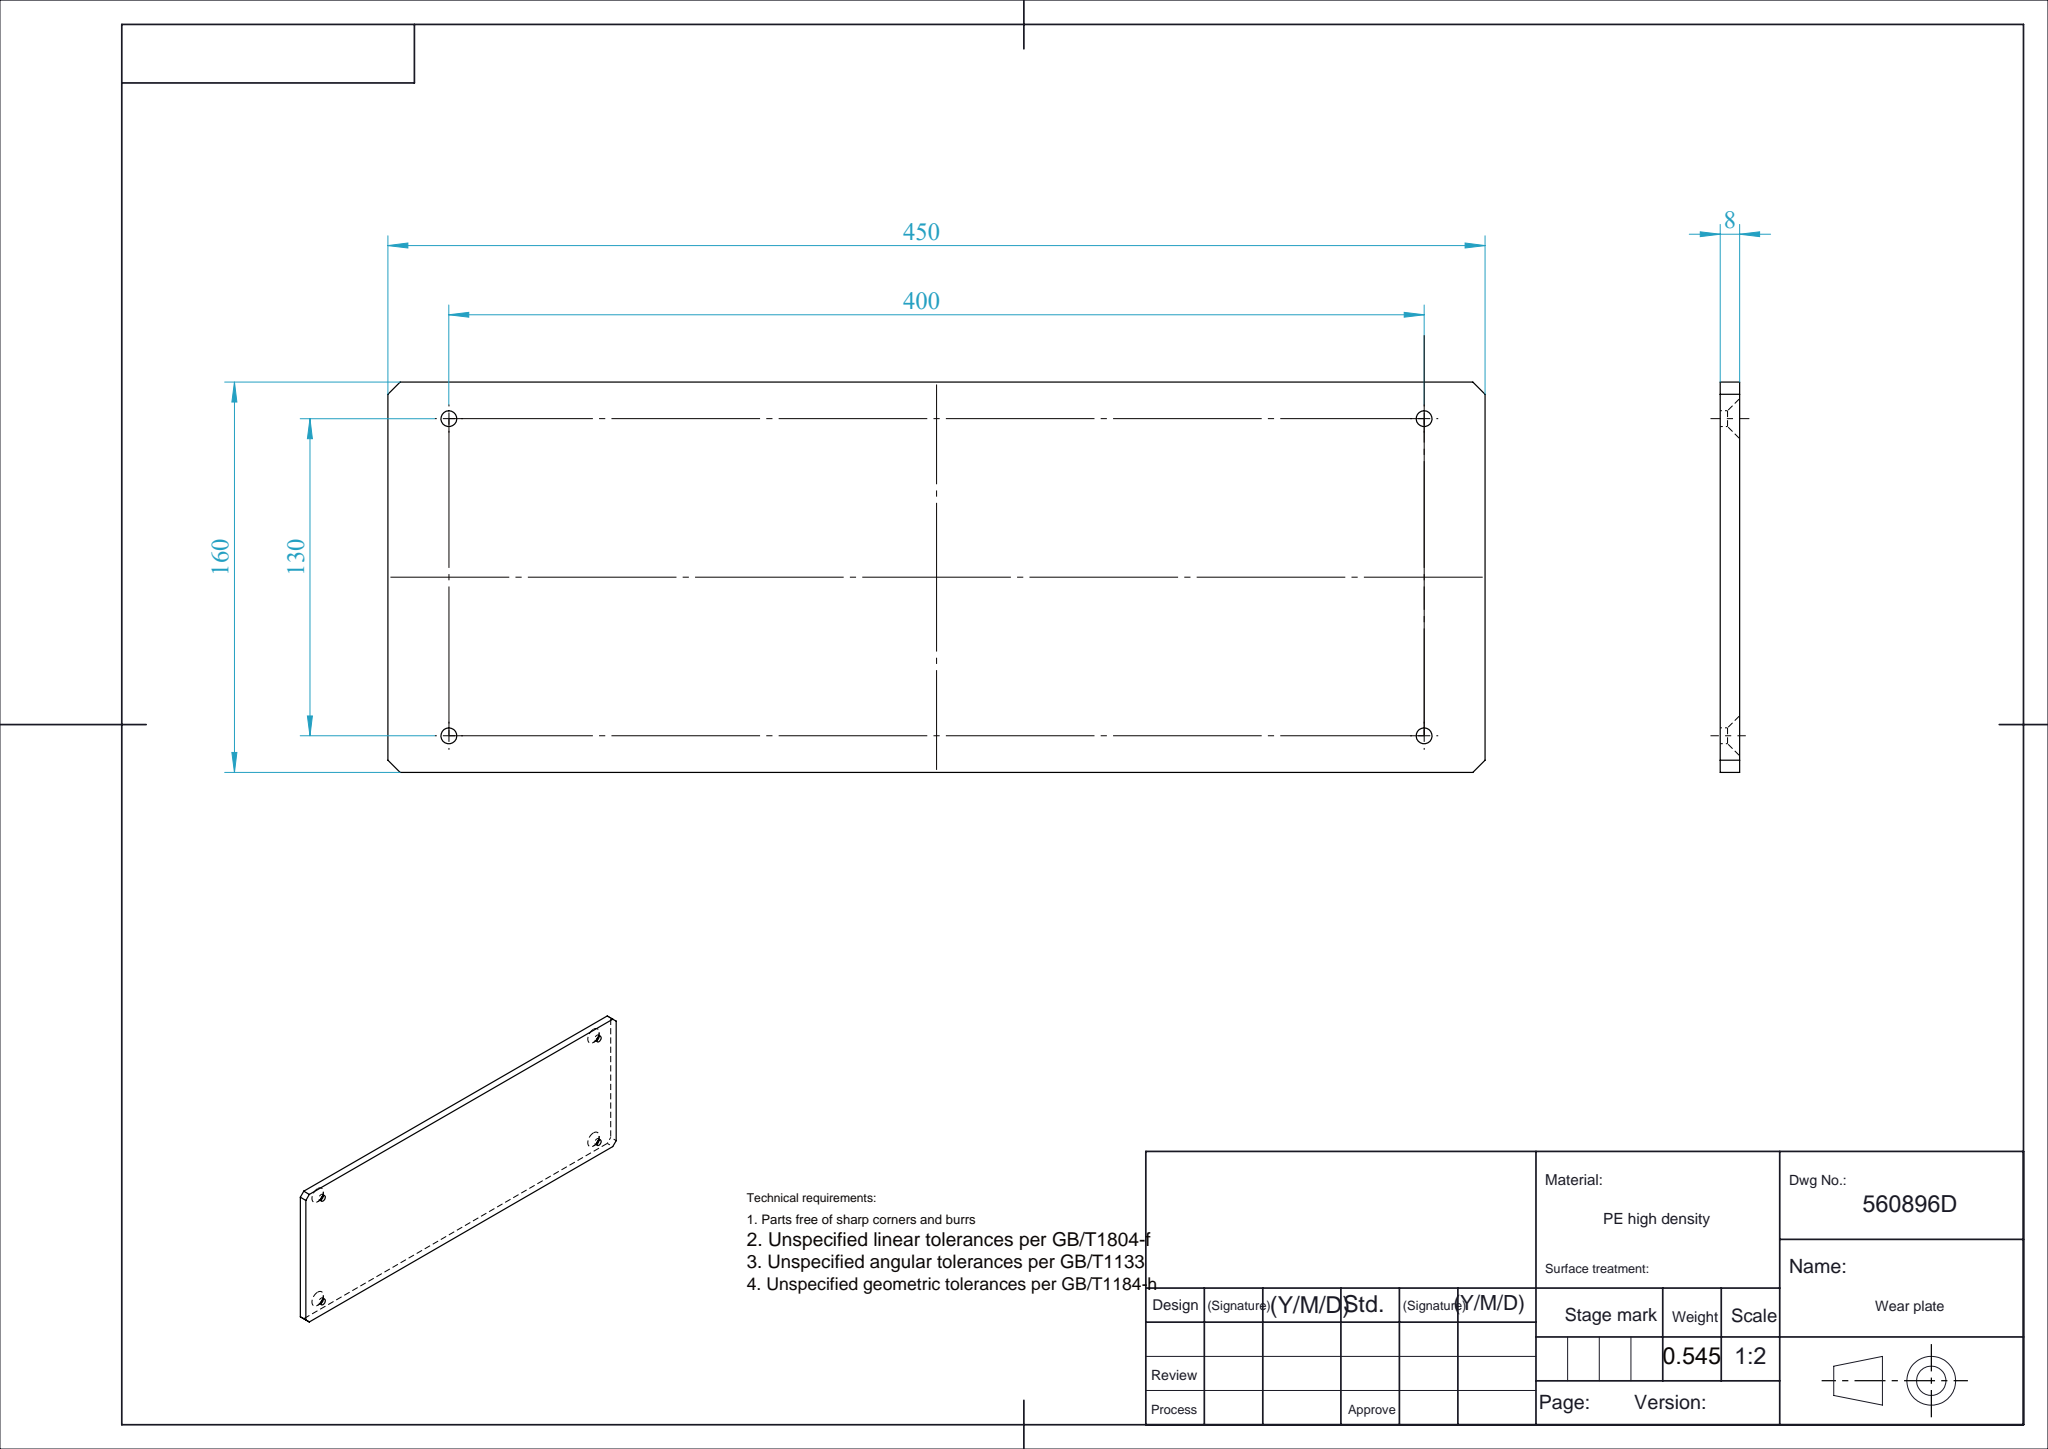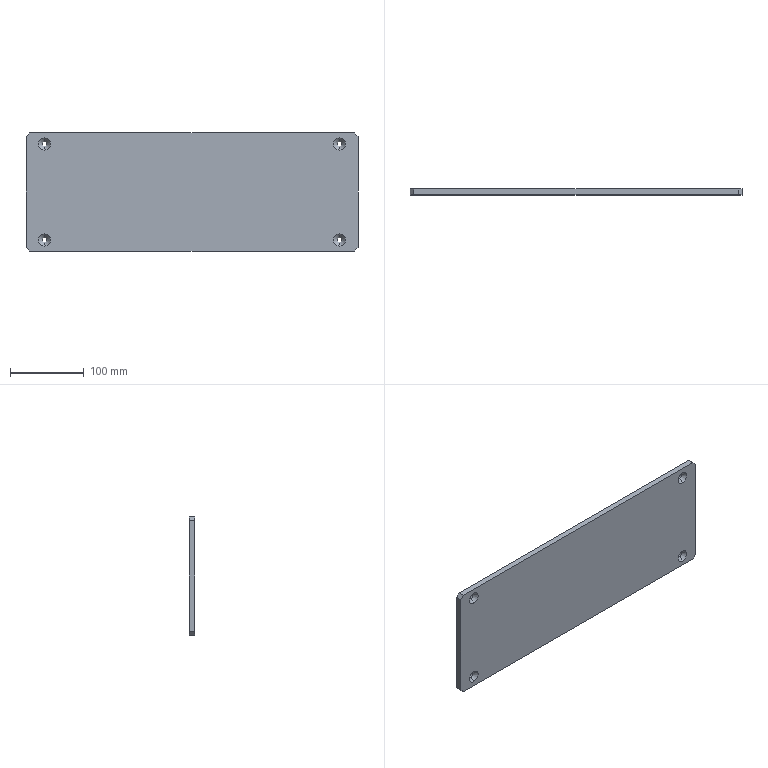Part | SolidWorks | features ICE 2, Chamfer 1, Extrusion 1 | 1 solid | 26 faces | box 450 x 8 x 160 mm | volume 572994 mm3 | plane 10 | cone 8 | cylinder 8 | commonest cylinder face diameters 6.5 x8
STEP:
#1=CARTESIAN_POINT('',(-200.,5.,68.25));
#2=VERTEX_POINT('',#1);
#3=CARTESIAN_POINT('',(-200.,5.,61.75));
#4=VERTEX_POINT('',#3);
#5=CARTESIAN_POINT('',(-200.,5.,65.));
#6=DIRECTION('',(0.,-1.,0.));
#7=DIRECTION('',(0.,0.,-1.));
#8=AXIS2_PLACEMENT_3D('',#5,#6,#7);
#9=CIRCLE('',#8,3.25);
#10=EDGE_CURVE('',#2,#4,#9,.T.);
#11=ORIENTED_EDGE('',*,*,#10,.F.);
#12=CARTESIAN_POINT('',(-200.,0.,73.25));
#13=VERTEX_POINT('',#12);
#14=CARTESIAN_POINT('',(-200.,0.,73.25));
#15=DIRECTION('',(0.,-0.7071,0.7071));
#16=VECTOR('',#15,1000.);
#17=LINE('',#14,#16);
#18=EDGE_CURVE('',#2,#13,#17,.T.);
#19=ORIENTED_EDGE('',*,*,#18,.T.);
#20=CARTESIAN_POINT('',(-200.,0.,56.75));
#21=VERTEX_POINT('',#20);
#22=CARTESIAN_POINT('',(-200.,0.,65.));
#23=DIRECTION('',(0.,-1.,0.));
#24=DIRECTION('',(0.,0.,-1.));
#25=AXIS2_PLACEMENT_3D('',#22,#23,#24);
#26=CIRCLE('',#25,8.25);
#27=EDGE_CURVE('',#13,#21,#26,.T.);
#28=ORIENTED_EDGE('',*,*,#27,.T.);
#29=CARTESIAN_POINT('',(-200.,0.,56.75));
#30=DIRECTION('',(0.,-0.7071,-0.7071));
#31=VECTOR('',#30,1000.);
#32=LINE('',#29,#31);
#33=EDGE_CURVE('',#4,#21,#32,.T.);
#34=ORIENTED_EDGE('',*,*,#33,.F.);
#35=EDGE_LOOP('',(#11,#19,#28,#34));
#36=FACE_OUTER_BOUND('',#35,.T.);
#37=CARTESIAN_POINT('',(-200.,0.,65.));
#38=DIRECTION('',(0.,-1.,0.));
#39=DIRECTION('',(0.,0.,-1.));
#40=AXIS2_PLACEMENT_3D('',#37,#38,#39);
#41=CONICAL_SURFACE('',#40,8.25,0.7854);
#42=ADVANCED_FACE('',(#36),#41,.F.);
#43=CARTESIAN_POINT('',(200.,5.,-61.75));
#44=VERTEX_POINT('',#43);
#45=CARTESIAN_POINT('',(200.,5.,-68.25));
#46=VERTEX_POINT('',#45);
#47=CARTESIAN_POINT('',(200.,5.,-65.));
#48=DIRECTION('',(0.,-1.,0.));
#49=DIRECTION('',(0.,0.,-1.));
#50=AXIS2_PLACEMENT_3D('',#47,#48,#49);
#51=CIRCLE('',#50,3.25);
#52=EDGE_CURVE('',#44,#46,#51,.T.);
#53=ORIENTED_EDGE('',*,*,#52,.F.);
#54=CARTESIAN_POINT('',(200.,0.,-56.75));
#55=VERTEX_POINT('',#54);
#56=CARTESIAN_POINT('',(200.,0.,-56.75));
#57=DIRECTION('',(0.,-0.7071,0.7071));
#58=VECTOR('',#57,1000.);
#59=LINE('',#56,#58);
#60=EDGE_CURVE('',#44,#55,#59,.T.);
#61=ORIENTED_EDGE('',*,*,#60,.T.);
#62=CARTESIAN_POINT('',(200.,0.,-73.25));
#63=VERTEX_POINT('',#62);
#64=CARTESIAN_POINT('',(200.,0.,-65.));
#65=DIRECTION('',(0.,-1.,0.));
#66=DIRECTION('',(0.,0.,-1.));
#67=AXIS2_PLACEMENT_3D('',#64,#65,#66);
#68=CIRCLE('',#67,8.25);
#69=EDGE_CURVE('',#55,#63,#68,.T.);
#70=ORIENTED_EDGE('',*,*,#69,.T.);
#71=CARTESIAN_POINT('',(200.,0.,-73.25));
#72=DIRECTION('',(0.,-0.7071,-0.7071));
#73=VECTOR('',#72,1000.);
#74=LINE('',#71,#73);
#75=EDGE_CURVE('',#46,#63,#74,.T.);
#76=ORIENTED_EDGE('',*,*,#75,.F.);
#77=EDGE_LOOP('',(#53,#61,#70,#76));
#78=FACE_OUTER_BOUND('',#77,.T.);
#79=CARTESIAN_POINT('',(200.,0.,-65.));
#80=DIRECTION('',(0.,-1.,0.));
#81=DIRECTION('',(0.,0.,-1.));
#82=AXIS2_PLACEMENT_3D('',#79,#80,#81);
#83=CONICAL_SURFACE('',#82,8.25,0.7854);
#84=ADVANCED_FACE('',(#78),#83,.F.);
#85=CARTESIAN_POINT('',(200.,5.,68.25));
#86=VERTEX_POINT('',#85);
#87=CARTESIAN_POINT('',(200.,5.,61.75));
#88=VERTEX_POINT('',#87);
#89=CARTESIAN_POINT('',(200.,5.,65.));
#90=DIRECTION('',(0.,-1.,0.));
#91=DIRECTION('',(0.,0.,-1.));
#92=AXIS2_PLACEMENT_3D('',#89,#90,#91);
#93=CIRCLE('',#92,3.25);
#94=EDGE_CURVE('',#86,#88,#93,.T.);
#95=ORIENTED_EDGE('',*,*,#94,.F.);
#96=CARTESIAN_POINT('',(200.,0.,73.25));
#97=VERTEX_POINT('',#96);
#98=CARTESIAN_POINT('',(200.,0.,73.25));
#99=DIRECTION('',(0.,-0.7071,0.7071));
#100=VECTOR('',#99,1000.);
#101=LINE('',#98,#100);
#102=EDGE_CURVE('',#86,#97,#101,.T.);
#103=ORIENTED_EDGE('',*,*,#102,.T.);
#104=CARTESIAN_POINT('',(200.,0.,56.75));
#105=VERTEX_POINT('',#104);
#106=CARTESIAN_POINT('',(200.,0.,65.));
#107=DIRECTION('',(0.,-1.,0.));
#108=DIRECTION('',(0.,0.,-1.));
#109=AXIS2_PLACEMENT_3D('',#106,#107,#108);
#110=CIRCLE('',#109,8.25);
#111=EDGE_CURVE('',#97,#105,#110,.T.);
#112=ORIENTED_EDGE('',*,*,#111,.T.);
#113=CARTESIAN_POINT('',(200.,0.,56.75));
#114=DIRECTION('',(0.,-0.7071,-0.7071));
#115=VECTOR('',#114,1000.);
#116=LINE('',#113,#115);
#117=EDGE_CURVE('',#88,#105,#116,.T.);
#118=ORIENTED_EDGE('',*,*,#117,.F.);
#119=EDGE_LOOP('',(#95,#103,#112,#118));
#120=FACE_OUTER_BOUND('',#119,.T.);
#121=CARTESIAN_POINT('',(200.,0.,65.));
#122=DIRECTION('',(0.,-1.,0.));
#123=DIRECTION('',(0.,0.,-1.));
#124=AXIS2_PLACEMENT_3D('',#121,#122,#123);
#125=CONICAL_SURFACE('',#124,8.25,0.7854);
#126=ADVANCED_FACE('',(#120),#125,.F.);
#127=CARTESIAN_POINT('',(-200.,5.,-61.75));
#128=VERTEX_POINT('',#127);
#129=CARTESIAN_POINT('',(-200.,5.,-68.25));
#130=VERTEX_POINT('',#129);
#131=CARTESIAN_POINT('',(-200.,5.,-65.));
#132=DIRECTION('',(0.,-1.,0.));
#133=DIRECTION('',(0.,0.,-1.));
#134=AXIS2_PLACEMENT_3D('',#131,#132,#133);
#135=CIRCLE('',#134,3.25);
#136=EDGE_CURVE('',#128,#130,#135,.T.);
#137=ORIENTED_EDGE('',*,*,#136,.F.);
#138=CARTESIAN_POINT('',(-200.,0.,-56.75));
#139=VERTEX_POINT('',#138);
#140=CARTESIAN_POINT('',(-200.,0.,-56.75));
#141=DIRECTION('',(0.,-0.7071,0.7071));
#142=VECTOR('',#141,1000.);
#143=LINE('',#140,#142);
#144=EDGE_CURVE('',#128,#139,#143,.T.);
#145=ORIENTED_EDGE('',*,*,#144,.T.);
#146=CARTESIAN_POINT('',(-200.,0.,-73.25));
#147=VERTEX_POINT('',#146);
#148=CARTESIAN_POINT('',(-200.,0.,-65.));
#149=DIRECTION('',(0.,-1.,0.));
#150=DIRECTION('',(0.,0.,-1.));
#151=AXIS2_PLACEMENT_3D('',#148,#149,#150);
#152=CIRCLE('',#151,8.25);
#153=EDGE_CURVE('',#139,#147,#152,.T.);
#154=ORIENTED_EDGE('',*,*,#153,.T.);
#155=CARTESIAN_POINT('',(-200.,0.,-73.25));
#156=DIRECTION('',(0.,-0.7071,-0.7071));
#157=VECTOR('',#156,1000.);
#158=LINE('',#155,#157);
#159=EDGE_CURVE('',#130,#147,#158,.T.);
#160=ORIENTED_EDGE('',*,*,#159,.F.);
#161=EDGE_LOOP('',(#137,#145,#154,#160));
#162=FACE_OUTER_BOUND('',#161,.T.);
#163=CARTESIAN_POINT('',(-200.,0.,-65.));
#164=DIRECTION('',(0.,-1.,0.));
#165=DIRECTION('',(0.,0.,-1.));
#166=AXIS2_PLACEMENT_3D('',#163,#164,#165);
#167=CONICAL_SURFACE('',#166,8.25,0.7854);
#168=ADVANCED_FACE('',(#162),#167,.F.);
#169=CARTESIAN_POINT('',(-200.,8.,-61.75));
#170=VERTEX_POINT('',#169);
#171=CARTESIAN_POINT('',(-200.,8.,-68.25));
#172=VERTEX_POINT('',#171);
#173=CARTESIAN_POINT('',(-200.,8.,-65.));
#174=DIRECTION('',(0.,-1.,0.));
#175=DIRECTION('',(0.,0.,-1.));
#176=AXIS2_PLACEMENT_3D('',#173,#174,#175);
#177=CIRCLE('',#176,3.25);
#178=EDGE_CURVE('',#170,#172,#177,.T.);
#179=ORIENTED_EDGE('',*,*,#178,.F.);
#180=CARTESIAN_POINT('',(-200.,8.,-61.75));
#181=DIRECTION('',(0.,-1.,0.));
#182=VECTOR('',#181,1000.);
#183=LINE('',#180,#182);
#184=EDGE_CURVE('',#170,#128,#183,.T.);
#185=ORIENTED_EDGE('',*,*,#184,.T.);
#186=ORIENTED_EDGE('',*,*,#136,.T.);
#187=CARTESIAN_POINT('',(-200.,8.,-68.25));
#188=DIRECTION('',(0.,-1.,0.));
#189=VECTOR('',#188,1000.);
#190=LINE('',#187,#189);
#191=EDGE_CURVE('',#172,#130,#190,.T.);
#192=ORIENTED_EDGE('',*,*,#191,.F.);
#193=EDGE_LOOP('',(#179,#185,#186,#192));
#194=FACE_OUTER_BOUND('',#193,.T.);
#195=CARTESIAN_POINT('',(-200.,8.,-65.));
#196=DIRECTION('',(0.,-1.,0.));
#197=DIRECTION('',(0.,0.,-1.));
#198=AXIS2_PLACEMENT_3D('',#195,#196,#197);
#199=CYLINDRICAL_SURFACE('',#198,3.25);
#200=ADVANCED_FACE('',(#194),#199,.F.);
#201=CARTESIAN_POINT('',(200.,8.,68.25));
#202=VERTEX_POINT('',#201);
#203=CARTESIAN_POINT('',(200.,8.,61.75));
#204=VERTEX_POINT('',#203);
#205=CARTESIAN_POINT('',(200.,8.,65.));
#206=DIRECTION('',(0.,-1.,0.));
#207=DIRECTION('',(0.,0.,-1.));
#208=AXIS2_PLACEMENT_3D('',#205,#206,#207);
#209=CIRCLE('',#208,3.25);
#210=EDGE_CURVE('',#202,#204,#209,.T.);
#211=ORIENTED_EDGE('',*,*,#210,.F.);
#212=CARTESIAN_POINT('',(200.,8.,68.25));
#213=DIRECTION('',(0.,-1.,0.));
#214=VECTOR('',#213,1000.);
#215=LINE('',#212,#214);
#216=EDGE_CURVE('',#202,#86,#215,.T.);
#217=ORIENTED_EDGE('',*,*,#216,.T.);
#218=ORIENTED_EDGE('',*,*,#94,.T.);
#219=CARTESIAN_POINT('',(200.,8.,61.75));
#220=DIRECTION('',(0.,-1.,0.));
#221=VECTOR('',#220,1000.);
#222=LINE('',#219,#221);
#223=EDGE_CURVE('',#204,#88,#222,.T.);
#224=ORIENTED_EDGE('',*,*,#223,.F.);
#225=EDGE_LOOP('',(#211,#217,#218,#224));
#226=FACE_OUTER_BOUND('',#225,.T.);
#227=CARTESIAN_POINT('',(200.,8.,65.));
#228=DIRECTION('',(0.,-1.,0.));
#229=DIRECTION('',(0.,0.,-1.));
#230=AXIS2_PLACEMENT_3D('',#227,#228,#229);
#231=CYLINDRICAL_SURFACE('',#230,3.25);
#232=ADVANCED_FACE('',(#226),#231,.F.);
#233=CARTESIAN_POINT('',(200.,8.,-61.75));
#234=VERTEX_POINT('',#233);
#235=CARTESIAN_POINT('',(200.,8.,-68.25));
#236=VERTEX_POINT('',#235);
#237=CARTESIAN_POINT('',(200.,8.,-65.));
#238=DIRECTION('',(0.,-1.,0.));
#239=DIRECTION('',(0.,0.,-1.));
#240=AXIS2_PLACEMENT_3D('',#237,#238,#239);
#241=CIRCLE('',#240,3.25);
#242=EDGE_CURVE('',#234,#236,#241,.T.);
#243=ORIENTED_EDGE('',*,*,#242,.F.);
#244=CARTESIAN_POINT('',(200.,8.,-61.75));
#245=DIRECTION('',(0.,-1.,0.));
#246=VECTOR('',#245,1000.);
#247=LINE('',#244,#246);
#248=EDGE_CURVE('',#234,#44,#247,.T.);
#249=ORIENTED_EDGE('',*,*,#248,.T.);
#250=ORIENTED_EDGE('',*,*,#52,.T.);
#251=CARTESIAN_POINT('',(200.,8.,-68.25));
#252=DIRECTION('',(0.,-1.,0.));
#253=VECTOR('',#252,1000.);
#254=LINE('',#251,#253);
#255=EDGE_CURVE('',#236,#46,#254,.T.);
#256=ORIENTED_EDGE('',*,*,#255,.F.);
#257=EDGE_LOOP('',(#243,#249,#250,#256));
#258=FACE_OUTER_BOUND('',#257,.T.);
#259=CARTESIAN_POINT('',(200.,8.,-65.));
#260=DIRECTION('',(0.,-1.,0.));
#261=DIRECTION('',(0.,0.,-1.));
#262=AXIS2_PLACEMENT_3D('',#259,#260,#261);
#263=CYLINDRICAL_SURFACE('',#262,3.25);
#264=ADVANCED_FACE('',(#258),#263,.F.);
#265=CARTESIAN_POINT('',(-200.,8.,68.25));
#266=VERTEX_POINT('',#265);
#267=CARTESIAN_POINT('',(-200.,8.,61.75));
#268=VERTEX_POINT('',#267);
#269=CARTESIAN_POINT('',(-200.,8.,65.));
#270=DIRECTION('',(0.,-1.,0.));
#271=DIRECTION('',(0.,0.,-1.));
#272=AXIS2_PLACEMENT_3D('',#269,#270,#271);
#273=CIRCLE('',#272,3.25);
#274=EDGE_CURVE('',#266,#268,#273,.T.);
#275=ORIENTED_EDGE('',*,*,#274,.F.);
#276=CARTESIAN_POINT('',(-200.,8.,68.25));
#277=DIRECTION('',(0.,-1.,0.));
#278=VECTOR('',#277,1000.);
#279=LINE('',#276,#278);
#280=EDGE_CURVE('',#266,#2,#279,.T.);
#281=ORIENTED_EDGE('',*,*,#280,.T.);
#282=ORIENTED_EDGE('',*,*,#10,.T.);
#283=CARTESIAN_POINT('',(-200.,8.,61.75));
#284=DIRECTION('',(0.,-1.,0.));
#285=VECTOR('',#284,1000.);
#286=LINE('',#283,#285);
#287=EDGE_CURVE('',#268,#4,#286,.T.);
#288=ORIENTED_EDGE('',*,*,#287,.F.);
#289=EDGE_LOOP('',(#275,#281,#282,#288));
#290=FACE_OUTER_BOUND('',#289,.T.);
#291=CARTESIAN_POINT('',(-200.,8.,65.));
#292=DIRECTION('',(0.,-1.,0.));
#293=DIRECTION('',(0.,0.,-1.));
#294=AXIS2_PLACEMENT_3D('',#291,#292,#293);
#295=CYLINDRICAL_SURFACE('',#294,3.25);
#296=ADVANCED_FACE('',(#290),#295,.F.);
#297=ORIENTED_EDGE('',*,*,#280,.F.);
#298=CARTESIAN_POINT('',(-200.,8.,65.));
#299=DIRECTION('',(0.,-1.,0.));
#300=DIRECTION('',(0.,0.,-1.));
#301=AXIS2_PLACEMENT_3D('',#298,#299,#300);
#302=CIRCLE('',#301,3.25);
#303=EDGE_CURVE('',#268,#266,#302,.T.);
#304=ORIENTED_EDGE('',*,*,#303,.F.);
#305=ORIENTED_EDGE('',*,*,#287,.T.);
#306=CARTESIAN_POINT('',(-200.,5.,65.));
#307=DIRECTION('',(0.,-1.,0.));
#308=DIRECTION('',(0.,0.,-1.));
#309=AXIS2_PLACEMENT_3D('',#306,#307,#308);
#310=CIRCLE('',#309,3.25);
#311=EDGE_CURVE('',#4,#2,#310,.T.);
#312=ORIENTED_EDGE('',*,*,#311,.T.);
#313=EDGE_LOOP('',(#297,#304,#305,#312));
#314=FACE_OUTER_BOUND('',#313,.T.);
#315=CARTESIAN_POINT('',(-200.,8.,65.));
#316=DIRECTION('',(0.,-1.,0.));
#317=DIRECTION('',(0.,0.,-1.));
#318=AXIS2_PLACEMENT_3D('',#315,#316,#317);
#319=CYLINDRICAL_SURFACE('',#318,3.25);
#320=ADVANCED_FACE('',(#314),#319,.F.);
#321=ORIENTED_EDGE('',*,*,#248,.F.);
#322=CARTESIAN_POINT('',(200.,8.,-65.));
#323=DIRECTION('',(0.,-1.,0.));
#324=DIRECTION('',(0.,0.,-1.));
#325=AXIS2_PLACEMENT_3D('',#322,#323,#324);
#326=CIRCLE('',#325,3.25);
#327=EDGE_CURVE('',#236,#234,#326,.T.);
#328=ORIENTED_EDGE('',*,*,#327,.F.);
#329=ORIENTED_EDGE('',*,*,#255,.T.);
#330=CARTESIAN_POINT('',(200.,5.,-65.));
#331=DIRECTION('',(0.,-1.,0.));
#332=DIRECTION('',(0.,0.,-1.));
#333=AXIS2_PLACEMENT_3D('',#330,#331,#332);
#334=CIRCLE('',#333,3.25);
#335=EDGE_CURVE('',#46,#44,#334,.T.);
#336=ORIENTED_EDGE('',*,*,#335,.T.);
#337=EDGE_LOOP('',(#321,#328,#329,#336));
#338=FACE_OUTER_BOUND('',#337,.T.);
#339=CARTESIAN_POINT('',(200.,8.,-65.));
#340=DIRECTION('',(0.,-1.,0.));
#341=DIRECTION('',(0.,0.,-1.));
#342=AXIS2_PLACEMENT_3D('',#339,#340,#341);
#343=CYLINDRICAL_SURFACE('',#342,3.25);
#344=ADVANCED_FACE('',(#338),#343,.F.);
#345=ORIENTED_EDGE('',*,*,#216,.F.);
#346=CARTESIAN_POINT('',(200.,8.,65.));
#347=DIRECTION('',(0.,-1.,0.));
#348=DIRECTION('',(0.,0.,-1.));
#349=AXIS2_PLACEMENT_3D('',#346,#347,#348);
#350=CIRCLE('',#349,3.25);
#351=EDGE_CURVE('',#204,#202,#350,.T.);
#352=ORIENTED_EDGE('',*,*,#351,.F.);
#353=ORIENTED_EDGE('',*,*,#223,.T.);
#354=CARTESIAN_POINT('',(200.,5.,65.));
#355=DIRECTION('',(0.,-1.,0.));
#356=DIRECTION('',(0.,0.,-1.));
#357=AXIS2_PLACEMENT_3D('',#354,#355,#356);
#358=CIRCLE('',#357,3.25);
#359=EDGE_CURVE('',#88,#86,#358,.T.);
#360=ORIENTED_EDGE('',*,*,#359,.T.);
#361=EDGE_LOOP('',(#345,#352,#353,#360));
#362=FACE_OUTER_BOUND('',#361,.T.);
#363=CARTESIAN_POINT('',(200.,8.,65.));
#364=DIRECTION('',(0.,-1.,0.));
#365=DIRECTION('',(0.,0.,-1.));
#366=AXIS2_PLACEMENT_3D('',#363,#364,#365);
#367=CYLINDRICAL_SURFACE('',#366,3.25);
#368=ADVANCED_FACE('',(#362),#367,.F.);
#369=ORIENTED_EDGE('',*,*,#184,.F.);
#370=CARTESIAN_POINT('',(-200.,8.,-65.));
#371=DIRECTION('',(0.,-1.,0.));
#372=DIRECTION('',(0.,0.,-1.));
#373=AXIS2_PLACEMENT_3D('',#370,#371,#372);
#374=CIRCLE('',#373,3.25);
#375=EDGE_CURVE('',#172,#170,#374,.T.);
#376=ORIENTED_EDGE('',*,*,#375,.F.);
#377=ORIENTED_EDGE('',*,*,#191,.T.);
#378=CARTESIAN_POINT('',(-200.,5.,-65.));
#379=DIRECTION('',(0.,-1.,0.));
#380=DIRECTION('',(0.,0.,-1.));
#381=AXIS2_PLACEMENT_3D('',#378,#379,#380);
#382=CIRCLE('',#381,3.25);
#383=EDGE_CURVE('',#130,#128,#382,.T.);
#384=ORIENTED_EDGE('',*,*,#383,.T.);
#385=EDGE_LOOP('',(#369,#376,#377,#384));
#386=FACE_OUTER_BOUND('',#385,.T.);
#387=CARTESIAN_POINT('',(-200.,8.,-65.));
#388=DIRECTION('',(0.,-1.,0.));
#389=DIRECTION('',(0.,0.,-1.));
#390=AXIS2_PLACEMENT_3D('',#387,#388,#389);
#391=CYLINDRICAL_SURFACE('',#390,3.25);
#392=ADVANCED_FACE('',(#386),#391,.F.);
#393=CARTESIAN_POINT('',(225.,0.,75.));
#394=VERTEX_POINT('',#393);
#395=CARTESIAN_POINT('',(225.,0.,-75.));
#396=VERTEX_POINT('',#395);
#397=CARTESIAN_POINT('',(225.,0.,-80.));
#398=DIRECTION('',(0.,0.,-1.));
#399=VECTOR('',#398,1000.);
#400=LINE('',#397,#399);
#401=EDGE_CURVE('',#394,#396,#400,.T.);
#402=ORIENTED_EDGE('',*,*,#401,.T.);
#403=CARTESIAN_POINT('',(225.,8.,-75.));
#404=VERTEX_POINT('',#403);
#405=CARTESIAN_POINT('',(225.,8.,-75.));
#406=DIRECTION('',(0.,1.,0.));
#407=VECTOR('',#406,1000.);
#408=LINE('',#405,#407);
#409=EDGE_CURVE('',#396,#404,#408,.T.);
#410=ORIENTED_EDGE('',*,*,#409,.T.);
#411=CARTESIAN_POINT('',(225.,8.,75.));
#412=VERTEX_POINT('',#411);
#413=CARTESIAN_POINT('',(225.,8.,-80.));
#414=DIRECTION('',(0.,0.,-1.));
#415=VECTOR('',#414,1000.);
#416=LINE('',#413,#415);
#417=EDGE_CURVE('',#412,#404,#416,.T.);
#418=ORIENTED_EDGE('',*,*,#417,.F.);
#419=CARTESIAN_POINT('',(225.,8.,75.));
#420=DIRECTION('',(0.,-1.,0.));
#421=VECTOR('',#420,1000.);
#422=LINE('',#419,#421);
#423=EDGE_CURVE('',#412,#394,#422,.T.);
#424=ORIENTED_EDGE('',*,*,#423,.T.);
#425=EDGE_LOOP('',(#402,#410,#418,#424));
#426=FACE_OUTER_BOUND('',#425,.T.);
#427=CARTESIAN_POINT('',(225.,8.,-80.));
#428=DIRECTION('',(-1.,0.,0.));
#429=DIRECTION('',(0.,0.,1.));
#430=AXIS2_PLACEMENT_3D('',#427,#428,#429);
#431=PLANE('',#430);
#432=ADVANCED_FACE('',(#426),#431,.F.);
#433=CARTESIAN_POINT('',(220.,8.,-80.));
#434=VERTEX_POINT('',#433);
#435=CARTESIAN_POINT('',(-220.,8.,-80.));
#436=VERTEX_POINT('',#435);
#437=CARTESIAN_POINT('',(-225.,8.,-80.));
#438=DIRECTION('',(-1.,0.,0.));
#439=VECTOR('',#438,1000.);
#440=LINE('',#437,#439);
#441=EDGE_CURVE('',#434,#436,#440,.T.);
#442=ORIENTED_EDGE('',*,*,#441,.F.);
#443=CARTESIAN_POINT('',(220.,0.,-80.));
#444=VERTEX_POINT('',#443);
#445=CARTESIAN_POINT('',(220.,8.,-80.));
#446=DIRECTION('',(0.,-1.,0.));
#447=VECTOR('',#446,1000.);
#448=LINE('',#445,#447);
#449=EDGE_CURVE('',#434,#444,#448,.T.);
#450=ORIENTED_EDGE('',*,*,#449,.T.);
#451=CARTESIAN_POINT('',(-220.,0.,-80.));
#452=VERTEX_POINT('',#451);
#453=CARTESIAN_POINT('',(-225.,0.,-80.));
#454=DIRECTION('',(-1.,0.,0.));
#455=VECTOR('',#454,1000.);
#456=LINE('',#453,#455);
#457=EDGE_CURVE('',#444,#452,#456,.T.);
#458=ORIENTED_EDGE('',*,*,#457,.T.);
#459=CARTESIAN_POINT('',(-220.,8.,-80.));
#460=DIRECTION('',(0.,1.,0.));
#461=VECTOR('',#460,1000.);
#462=LINE('',#459,#461);
#463=EDGE_CURVE('',#452,#436,#462,.T.);
#464=ORIENTED_EDGE('',*,*,#463,.T.);
#465=EDGE_LOOP('',(#442,#450,#458,#464));
#466=FACE_OUTER_BOUND('',#465,.T.);
#467=CARTESIAN_POINT('',(-225.,8.,-80.));
#468=DIRECTION('',(0.,0.,1.));
#469=DIRECTION('',(1.,0.,0.));
#470=AXIS2_PLACEMENT_3D('',#467,#468,#469);
#471=PLANE('',#470);
#472=ADVANCED_FACE('',(#466),#471,.F.);
#473=CARTESIAN_POINT('',(-225.,8.,-75.));
#474=VERTEX_POINT('',#473);
#475=CARTESIAN_POINT('',(-225.,8.,75.));
#476=VERTEX_POINT('',#475);
#477=CARTESIAN_POINT('',(-225.,8.,-80.));
#478=DIRECTION('',(0.,0.,1.));
#479=VECTOR('',#478,1000.);
#480=LINE('',#477,#479);
#481=EDGE_CURVE('',#474,#476,#480,.T.);
#482=ORIENTED_EDGE('',*,*,#481,.F.);
#483=CARTESIAN_POINT('',(-225.,0.,-75.));
#484=VERTEX_POINT('',#483);
#485=CARTESIAN_POINT('',(-225.,8.,-75.));
#486=DIRECTION('',(0.,-1.,0.));
#487=VECTOR('',#486,1000.);
#488=LINE('',#485,#487);
#489=EDGE_CURVE('',#474,#484,#488,.T.);
#490=ORIENTED_EDGE('',*,*,#489,.T.);
#491=CARTESIAN_POINT('',(-225.,0.,75.));
#492=VERTEX_POINT('',#491);
#493=CARTESIAN_POINT('',(-225.,0.,-80.));
#494=DIRECTION('',(0.,0.,1.));
#495=VECTOR('',#494,1000.);
#496=LINE('',#493,#495);
#497=EDGE_CURVE('',#484,#492,#496,.T.);
#498=ORIENTED_EDGE('',*,*,#497,.T.);
#499=CARTESIAN_POINT('',(-225.,8.,75.));
#500=DIRECTION('',(0.,1.,0.));
#501=VECTOR('',#500,1000.);
#502=LINE('',#499,#501);
#503=EDGE_CURVE('',#492,#476,#502,.T.);
#504=ORIENTED_EDGE('',*,*,#503,.T.);
#505=EDGE_LOOP('',(#482,#490,#498,#504));
#506=FACE_OUTER_BOUND('',#505,.T.);
#507=CARTESIAN_POINT('',(-225.,8.,-80.));
#508=DIRECTION('',(1.,0.,0.));
#509=DIRECTION('',(0.,0.,-1.));
#510=AXIS2_PLACEMENT_3D('',#507,#508,#509);
#511=PLANE('',#510);
#512=ADVANCED_FACE('',(#506),#511,.F.);
#513=CARTESIAN_POINT('',(-220.,0.,80.));
#514=VERTEX_POINT('',#513);
#515=CARTESIAN_POINT('',(220.,0.,80.));
#516=VERTEX_POINT('',#515);
#517=CARTESIAN_POINT('',(-225.,0.,80.));
#518=DIRECTION('',(1.,0.,0.));
#519=VECTOR('',#518,1000.);
#520=LINE('',#517,#519);
#521=EDGE_CURVE('',#514,#516,#520,.T.);
#522=ORIENTED_EDGE('',*,*,#521,.T.);
#523=CARTESIAN_POINT('',(220.,8.,80.));
#524=VERTEX_POINT('',#523);
#525=CARTESIAN_POINT('',(220.,8.,80.));
#526=DIRECTION('',(0.,1.,0.));
#527=VECTOR('',#526,1000.);
#528=LINE('',#525,#527);
#529=EDGE_CURVE('',#516,#524,#528,.T.);
#530=ORIENTED_EDGE('',*,*,#529,.T.);
#531=CARTESIAN_POINT('',(-220.,8.,80.));
#532=VERTEX_POINT('',#531);
#533=CARTESIAN_POINT('',(-225.,8.,80.));
#534=DIRECTION('',(1.,0.,0.));
#535=VECTOR('',#534,1000.);
#536=LINE('',#533,#535);
#537=EDGE_CURVE('',#532,#524,#536,.T.);
#538=ORIENTED_EDGE('',*,*,#537,.F.);
#539=CARTESIAN_POINT('',(-220.,8.,80.));
#540=DIRECTION('',(0.,-1.,0.));
#541=VECTOR('',#540,1000.);
#542=LINE('',#539,#541);
#543=EDGE_CURVE('',#532,#514,#542,.T.);
#544=ORIENTED_EDGE('',*,*,#543,.T.);
#545=EDGE_LOOP('',(#522,#530,#538,#544));
#546=FACE_OUTER_BOUND('',#545,.T.);
#547=CARTESIAN_POINT('',(-225.,8.,80.));
#548=DIRECTION('',(0.,0.,-1.));
#549=DIRECTION('',(-1.,0.,0.));
#550=AXIS2_PLACEMENT_3D('',#547,#548,#549);
#551=PLANE('',#550);
#552=ADVANCED_FACE('',(#546),#551,.F.);
#553=ORIENTED_EDGE('',*,*,#375,.T.);
#554=ORIENTED_EDGE('',*,*,#178,.T.);
#555=EDGE_LOOP('',(#553,#554));
#556=FACE_BOUND('',#555,.T.);
#557=ORIENTED_EDGE('',*,*,#351,.T.);
#558=ORIENTED_EDGE('',*,*,#210,.T.);
#559=EDGE_LOOP('',(#557,#558));
#560=FACE_BOUND('',#559,.T.);
#561=ORIENTED_EDGE('',*,*,#327,.T.);
#562=ORIENTED_EDGE('',*,*,#242,.T.);
#563=EDGE_LOOP('',(#561,#562));
#564=FACE_BOUND('',#563,.T.);
#565=ORIENTED_EDGE('',*,*,#303,.T.);
#566=ORIENTED_EDGE('',*,*,#274,.T.);
#567=EDGE_LOOP('',(#565,#566));
#568=FACE_BOUND('',#567,.T.);
#569=ORIENTED_EDGE('',*,*,#417,.T.);
#570=CARTESIAN_POINT('',(150.,8.,-150.));
#571=DIRECTION('',(-0.7071,0.,-0.7071));
#572=VECTOR('',#571,1000.);
#573=LINE('',#570,#572);
#574=EDGE_CURVE('',#404,#434,#573,.T.);
#575=ORIENTED_EDGE('',*,*,#574,.T.);
#576=ORIENTED_EDGE('',*,*,#441,.T.);
#577=CARTESIAN_POINT('',(-150.,8.,-150.));
#578=DIRECTION('',(-0.7071,0.,0.7071));
#579=VECTOR('',#578,1000.);
#580=LINE('',#577,#579);
#581=EDGE_CURVE('',#436,#474,#580,.T.);
#582=ORIENTED_EDGE('',*,*,#581,.T.);
#583=ORIENTED_EDGE('',*,*,#481,.T.);
#584=CARTESIAN_POINT('',(-150.,8.,150.));
#585=DIRECTION('',(0.7071,0.,0.7071));
#586=VECTOR('',#585,1000.);
#587=LINE('',#584,#586);
#588=EDGE_CURVE('',#476,#532,#587,.T.);
#589=ORIENTED_EDGE('',*,*,#588,.T.);
#590=ORIENTED_EDGE('',*,*,#537,.T.);
#591=CARTESIAN_POINT('',(150.,8.,150.));
#592=DIRECTION('',(0.7071,0.,-0.7071));
#593=VECTOR('',#592,1000.);
#594=LINE('',#591,#593);
#595=EDGE_CURVE('',#524,#412,#594,.T.);
#596=ORIENTED_EDGE('',*,*,#595,.T.);
#597=EDGE_LOOP('',(#569,#575,#576,#582,#583,#589,#590,#596));
#598=FACE_OUTER_BOUND('',#597,.T.);
#599=CARTESIAN_POINT('',(0.,8.,0.));
#600=DIRECTION('',(0.,1.,0.));
#601=DIRECTION('',(0.,0.,1.));
#602=AXIS2_PLACEMENT_3D('',#599,#600,#601);
#603=PLANE('',#602);
#604=ADVANCED_FACE('',(#556,#560,#564,#568,#598),#603,.T.);
#605=CARTESIAN_POINT('',(-200.,0.,-65.));
#606=DIRECTION('',(0.,-1.,0.));
#607=DIRECTION('',(0.,0.,-1.));
#608=AXIS2_PLACEMENT_3D('',#605,#606,#607);
#609=CIRCLE('',#608,8.25);
#610=EDGE_CURVE('',#147,#139,#609,.T.);
#611=ORIENTED_EDGE('',*,*,#610,.F.);
#612=ORIENTED_EDGE('',*,*,#153,.F.);
#613=EDGE_LOOP('',(#611,#612));
#614=FACE_BOUND('',#613,.T.);
#615=CARTESIAN_POINT('',(200.,0.,65.));
#616=DIRECTION('',(0.,-1.,0.));
#617=DIRECTION('',(0.,0.,-1.));
#618=AXIS2_PLACEMENT_3D('',#615,#616,#617);
#619=CIRCLE('',#618,8.25);
#620=EDGE_CURVE('',#105,#97,#619,.T.);
#621=ORIENTED_EDGE('',*,*,#620,.F.);
#622=ORIENTED_EDGE('',*,*,#111,.F.);
#623=EDGE_LOOP('',(#621,#622));
#624=FACE_BOUND('',#623,.T.);
#625=CARTESIAN_POINT('',(200.,0.,-65.));
#626=DIRECTION('',(0.,-1.,0.));
#627=DIRECTION('',(0.,0.,-1.));
#628=AXIS2_PLACEMENT_3D('',#625,#626,#627);
#629=CIRCLE('',#628,8.25);
#630=EDGE_CURVE('',#63,#55,#629,.T.);
#631=ORIENTED_EDGE('',*,*,#630,.F.);
#632=ORIENTED_EDGE('',*,*,#69,.F.);
#633=EDGE_LOOP('',(#631,#632));
#634=FACE_BOUND('',#633,.T.);
#635=CARTESIAN_POINT('',(-200.,0.,65.));
#636=DIRECTION('',(0.,-1.,0.));
#637=DIRECTION('',(0.,0.,-1.));
#638=AXIS2_PLACEMENT_3D('',#635,#636,#637);
#639=CIRCLE('',#638,8.25);
#640=EDGE_CURVE('',#21,#13,#639,.T.);
#641=ORIENTED_EDGE('',*,*,#640,.F.);
#642=ORIENTED_EDGE('',*,*,#27,.F.);
#643=EDGE_LOOP('',(#641,#642));
#644=FACE_BOUND('',#643,.T.);
#645=ORIENTED_EDGE('',*,*,#457,.F.);
#646=CARTESIAN_POINT('',(220.,0.,-80.));
#647=DIRECTION('',(0.7071,0.,0.7071));
#648=VECTOR('',#647,1000.);
#649=LINE('',#646,#648);
#650=EDGE_CURVE('',#444,#396,#649,.T.);
#651=ORIENTED_EDGE('',*,*,#650,.T.);
#652=ORIENTED_EDGE('',*,*,#401,.F.);
#653=CARTESIAN_POINT('',(225.,0.,75.));
#654=DIRECTION('',(-0.7071,0.,0.7071));
#655=VECTOR('',#654,1000.);
#656=LINE('',#653,#655);
#657=EDGE_CURVE('',#394,#516,#656,.T.);
#658=ORIENTED_EDGE('',*,*,#657,.T.);
#659=ORIENTED_EDGE('',*,*,#521,.F.);
#660=CARTESIAN_POINT('',(-220.,0.,80.));
#661=DIRECTION('',(-0.7071,0.,-0.7071));
#662=VECTOR('',#661,1000.);
#663=LINE('',#660,#662);
#664=EDGE_CURVE('',#514,#492,#663,.T.);
#665=ORIENTED_EDGE('',*,*,#664,.T.);
#666=ORIENTED_EDGE('',*,*,#497,.F.);
#667=CARTESIAN_POINT('',(-225.,0.,-75.));
#668=DIRECTION('',(0.7071,0.,-0.7071));
#669=VECTOR('',#668,1000.);
#670=LINE('',#667,#669);
#671=EDGE_CURVE('',#484,#452,#670,.T.);
#672=ORIENTED_EDGE('',*,*,#671,.T.);
#673=EDGE_LOOP('',(#645,#651,#652,#658,#659,#665,#666,#672));
#674=FACE_OUTER_BOUND('',#673,.T.);
#675=CARTESIAN_POINT('',(0.,0.,0.));
#676=DIRECTION('',(0.,1.,0.));
#677=DIRECTION('',(0.,0.,1.));
#678=AXIS2_PLACEMENT_3D('',#675,#676,#677);
#679=PLANE('',#678);
#680=ADVANCED_FACE('',(#614,#624,#634,#644,#674),#679,.F.);
#681=ORIENTED_EDGE('',*,*,#144,.F.);
#682=ORIENTED_EDGE('',*,*,#383,.F.);
#683=ORIENTED_EDGE('',*,*,#159,.T.);
#684=ORIENTED_EDGE('',*,*,#610,.T.);
#685=EDGE_LOOP('',(#681,#682,#683,#684));
#686=FACE_OUTER_BOUND('',#685,.T.);
#687=CARTESIAN_POINT('',(-200.,0.,-65.));
#688=DIRECTION('',(0.,-1.,0.));
#689=DIRECTION('',(0.,0.,-1.));
#690=AXIS2_PLACEMENT_3D('',#687,#688,#689);
#691=CONICAL_SURFACE('',#690,8.25,0.7854);
#692=ADVANCED_FACE('',(#686),#691,.F.);
#693=ORIENTED_EDGE('',*,*,#102,.F.);
#694=ORIENTED_EDGE('',*,*,#359,.F.);
#695=ORIENTED_EDGE('',*,*,#117,.T.);
#696=ORIENTED_EDGE('',*,*,#620,.T.);
#697=EDGE_LOOP('',(#693,#694,#695,#696));
#698=FACE_OUTER_BOUND('',#697,.T.);
#699=CARTESIAN_POINT('',(200.,0.,65.));
#700=DIRECTION('',(0.,-1.,0.));
#701=DIRECTION('',(0.,0.,-1.));
#702=AXIS2_PLACEMENT_3D('',#699,#700,#701);
#703=CONICAL_SURFACE('',#702,8.25,0.7854);
#704=ADVANCED_FACE('',(#698),#703,.F.);
#705=ORIENTED_EDGE('',*,*,#60,.F.);
#706=ORIENTED_EDGE('',*,*,#335,.F.);
#707=ORIENTED_EDGE('',*,*,#75,.T.);
#708=ORIENTED_EDGE('',*,*,#630,.T.);
#709=EDGE_LOOP('',(#705,#706,#707,#708));
#710=FACE_OUTER_BOUND('',#709,.T.);
#711=CARTESIAN_POINT('',(200.,0.,-65.));
#712=DIRECTION('',(0.,-1.,0.));
#713=DIRECTION('',(0.,0.,-1.));
#714=AXIS2_PLACEMENT_3D('',#711,#712,#713);
#715=CONICAL_SURFACE('',#714,8.25,0.7854);
#716=ADVANCED_FACE('',(#710),#715,.F.);
#717=ORIENTED_EDGE('',*,*,#18,.F.);
#718=ORIENTED_EDGE('',*,*,#311,.F.);
#719=ORIENTED_EDGE('',*,*,#33,.T.);
#720=ORIENTED_EDGE('',*,*,#640,.T.);
#721=EDGE_LOOP('',(#717,#718,#719,#720));
#722=FACE_OUTER_BOUND('',#721,.T.);
#723=CARTESIAN_POINT('',(-200.,0.,65.));
#724=DIRECTION('',(0.,-1.,0.));
#725=DIRECTION('',(0.,0.,-1.));
#726=AXIS2_PLACEMENT_3D('',#723,#724,#725);
#727=CONICAL_SURFACE('',#726,8.25,0.7854);
#728=ADVANCED_FACE('',(#722),#727,.F.);
#729=ORIENTED_EDGE('',*,*,#574,.F.);
#730=ORIENTED_EDGE('',*,*,#409,.F.);
#731=ORIENTED_EDGE('',*,*,#650,.F.);
#732=ORIENTED_EDGE('',*,*,#449,.F.);
#733=EDGE_LOOP('',(#729,#730,#731,#732));
#734=FACE_OUTER_BOUND('',#733,.T.);
#735=CARTESIAN_POINT('',(220.,8.,-80.));
#736=DIRECTION('',(-0.7071,0.,0.7071));
#737=DIRECTION('',(0.,-1.,0.));
#738=AXIS2_PLACEMENT_3D('',#735,#736,#737);
#739=PLANE('',#738);
#740=ADVANCED_FACE('',(#734),#739,.F.);
#741=ORIENTED_EDGE('',*,*,#595,.F.);
#742=ORIENTED_EDGE('',*,*,#529,.F.);
#743=ORIENTED_EDGE('',*,*,#657,.F.);
#744=ORIENTED_EDGE('',*,*,#423,.F.);
#745=EDGE_LOOP('',(#741,#742,#743,#744));
#746=FACE_OUTER_BOUND('',#745,.T.);
#747=CARTESIAN_POINT('',(225.,8.,75.));
#748=DIRECTION('',(-0.7071,0.,-0.7071));
#749=DIRECTION('',(0.,-1.,0.));
#750=AXIS2_PLACEMENT_3D('',#747,#748,#749);
#751=PLANE('',#750);
#752=ADVANCED_FACE('',(#746),#751,.F.);
#753=ORIENTED_EDGE('',*,*,#581,.F.);
#754=ORIENTED_EDGE('',*,*,#463,.F.);
#755=ORIENTED_EDGE('',*,*,#671,.F.);
#756=ORIENTED_EDGE('',*,*,#489,.F.);
#757=EDGE_LOOP('',(#753,#754,#755,#756));
#758=FACE_OUTER_BOUND('',#757,.T.);
#759=CARTESIAN_POINT('',(-225.,8.,-75.));
#760=DIRECTION('',(0.7071,0.,0.7071));
#761=DIRECTION('',(0.,-1.,0.));
#762=AXIS2_PLACEMENT_3D('',#759,#760,#761);
#763=PLANE('',#762);
#764=ADVANCED_FACE('',(#758),#763,.F.);
#765=ORIENTED_EDGE('',*,*,#588,.F.);
#766=ORIENTED_EDGE('',*,*,#503,.F.);
#767=ORIENTED_EDGE('',*,*,#664,.F.);
#768=ORIENTED_EDGE('',*,*,#543,.F.);
#769=EDGE_LOOP('',(#765,#766,#767,#768));
#770=FACE_OUTER_BOUND('',#769,.T.);
#771=CARTESIAN_POINT('',(-220.,8.,80.));
#772=DIRECTION('',(0.7071,0.,-0.7071));
#773=DIRECTION('',(0.,-1.,0.));
#774=AXIS2_PLACEMENT_3D('',#771,#772,#773);
#775=PLANE('',#774);
#776=ADVANCED_FACE('',(#770),#775,.F.);
#777=CLOSED_SHELL('',(#42,#84,#126,#168,#200,#232,#264,#296,#320,#344,#368,#392,#432,#472,#512,#552,#604,#680,#692,#704,#716,#728,#740,#752,#764,#776));
#778=MANIFOLD_SOLID_BREP('',#777);
#779=CARTESIAN_POINT('',(0.,0.,0.));
#780=DIRECTION('',(0.,0.,1.));
#781=DIRECTION('',(1.,0.,0.));
#782=AXIS2_PLACEMENT_3D('',#779,#780,#781);
#783=(LENGTH_UNIT()NAMED_UNIT(*)SI_UNIT(.MILLI.,.METRE.));
#784=UNCERTAINTY_MEASURE_WITH_UNIT(LENGTH_MEASURE(0.00001),#783,'','');
#785=(NAMED_UNIT(*)PLANE_ANGLE_UNIT()SI_UNIT($,.RADIAN.));
#786=(NAMED_UNIT(*)SI_UNIT($,.STERADIAN.)SOLID_ANGLE_UNIT());
#787=(GEOMETRIC_REPRESENTATION_CONTEXT(3)GLOBAL_UNCERTAINTY_ASSIGNED_CONTEXT((#784))GLOBAL_UNIT_ASSIGNED_CONTEXT((#783,#785,#786))REPRESENTATION_CONTEXT('',''));
#788=ADVANCED_BREP_SHAPE_REPRESENTATION('',(#778,#782),#787);